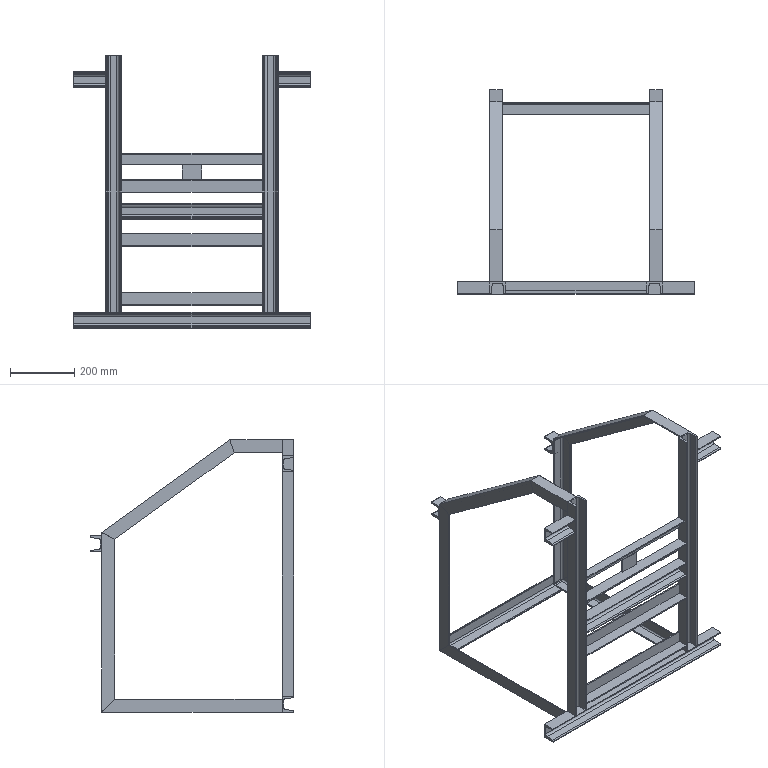Part | SolidWorks | features WeldMemberFeat 8, WeldCornerFeat 5, ICE 2, 3DProfileFeature 1, WeldmentFeature 1 | 22 solids | 257 faces | box 740 x 637 x 850 mm | volume 3794275 mm3 | plane 198 | cylinder 59 | commonest cylinder face diameters 2.667 x18 7 x16 14 x16 10 x9